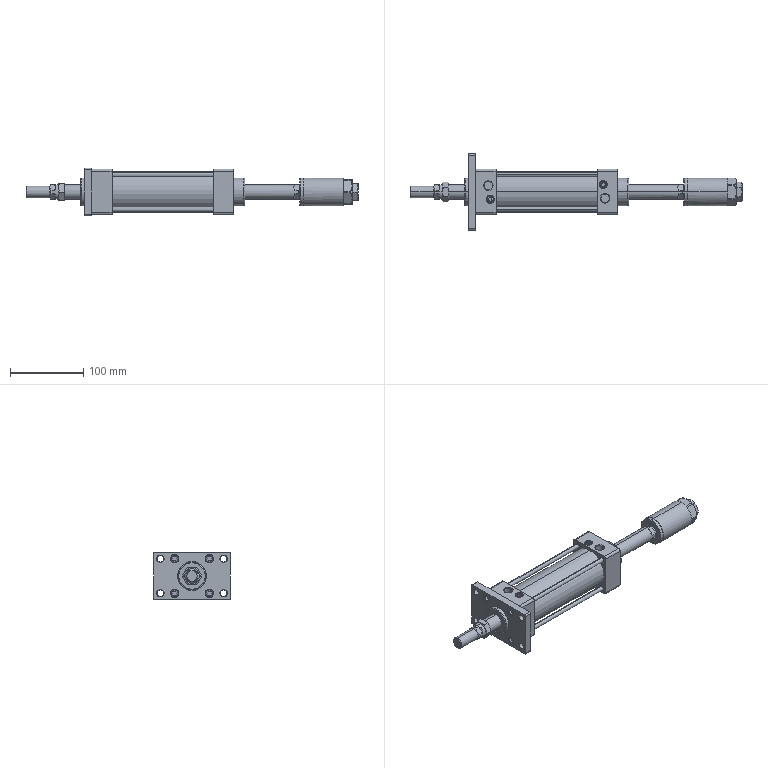Part | SolidWorks | features CompositeCurve 1 | 10 solids | 411 faces | box 452 x 104 x 65 mm | volume 566807 mm3 | cylinder 148 | plane 143 | cone 106 | torus 14 | commonest cylinder face diameters 6 x24 4.917 x16 9.5 x16 6.5 x8 9 x8 10 x8